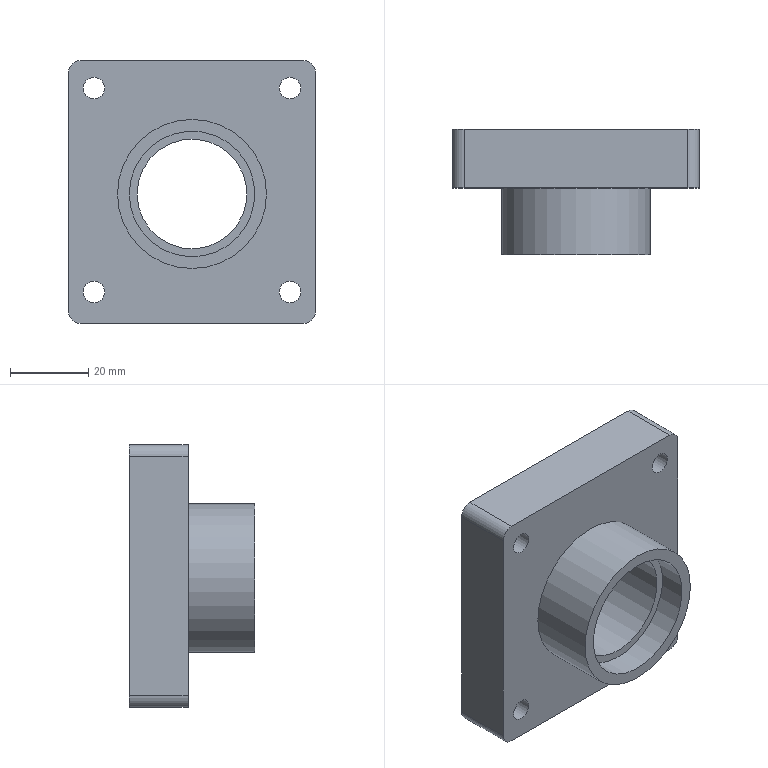Part | STEP file | ROTATION MC_NEW VER-0610_1021 | 1 solid | 29 faces | box 63 x 32 x 67 mm | volume 57913 mm3 | cylinder 16 | plane 13 | commonest cylinder face diameters 5.5 x4 6 x4 9 x4 32 x2 28 x1 38 x1
STEP:
#1=CARTESIAN_POINT('',(-200.969,622.268,-55.091));
#2=VERTEX_POINT('',#1);
#3=CARTESIAN_POINT('',(-203.969,622.268,-52.091));
#4=VERTEX_POINT('',#3);
#5=CARTESIAN_POINT('',(-203.969,622.268,-55.091));
#6=DIRECTION('',(0.,-1.,0.));
#7=DIRECTION('',(0.7071,0.,0.7071));
#8=AXIS2_PLACEMENT_3D('',#5,#6,#7);
#9=CIRCLE('',#8,3.);
#10=EDGE_CURVE('',#2,#4,#9,.T.);
#11=ORIENTED_EDGE('',*,*,#10,.T.);
#12=CARTESIAN_POINT('',(-203.969,607.268,-52.091));
#13=VERTEX_POINT('',#12);
#14=CARTESIAN_POINT('',(-203.969,604.268,-52.091));
#15=DIRECTION('',(0.,-1.,0.));
#16=VECTOR('',#15,10.);
#17=LINE('',#14,#16);
#18=EDGE_CURVE('',#4,#13,#17,.T.);
#19=ORIENTED_EDGE('',*,*,#18,.T.);
#20=CARTESIAN_POINT('',(-200.969,607.268,-55.091));
#21=VERTEX_POINT('',#20);
#22=CARTESIAN_POINT('',(-203.969,607.268,-55.091));
#23=DIRECTION('',(0.,1.,0.));
#24=DIRECTION('',(0.7071,0.,0.7071));
#25=AXIS2_PLACEMENT_3D('',#22,#23,#24);
#26=CIRCLE('',#25,3.);
#27=EDGE_CURVE('',#13,#21,#26,.T.);
#28=ORIENTED_EDGE('',*,*,#27,.T.);
#29=CARTESIAN_POINT('',(-200.969,604.268,-55.091));
#30=DIRECTION('',(0.,1.,0.));
#31=VECTOR('',#30,10.);
#32=LINE('',#29,#31);
#33=EDGE_CURVE('',#21,#2,#32,.T.);
#34=ORIENTED_EDGE('',*,*,#33,.T.);
#35=EDGE_LOOP('',(#11,#19,#28,#34));
#36=FACE_OUTER_BOUND('',#35,.T.);
#37=CARTESIAN_POINT('',(-203.969,604.268,-55.091));
#38=DIRECTION('',(0.,1.,0.));
#39=DIRECTION('',(0.7071,0.,0.7071));
#40=AXIS2_PLACEMENT_3D('',#37,#38,#39);
#41=CYLINDRICAL_SURFACE('',#40,3.);
#42=ADVANCED_FACE('',(#36),#41,.T.);
#43=ORIENTED_EDGE('',*,*,#33,.F.);
#44=CARTESIAN_POINT('',(-200.969,607.268,-116.091));
#45=VERTEX_POINT('',#44);
#46=CARTESIAN_POINT('',(-200.969,607.268,-47.091));
#47=DIRECTION('',(0.,0.,-1.));
#48=VECTOR('',#47,69.);
#49=LINE('',#46,#48);
#50=EDGE_CURVE('',#21,#45,#49,.T.);
#51=ORIENTED_EDGE('',*,*,#50,.T.);
#52=CARTESIAN_POINT('',(-200.969,622.268,-116.091));
#53=VERTEX_POINT('',#52);
#54=CARTESIAN_POINT('',(-200.969,622.268,-116.091));
#55=DIRECTION('',(0.,-1.,0.));
#56=VECTOR('',#55,10.);
#57=LINE('',#54,#56);
#58=EDGE_CURVE('',#45,#53,#57,.F.);
#59=ORIENTED_EDGE('',*,*,#58,.T.);
#60=CARTESIAN_POINT('',(-200.969,622.268,-47.091));
#61=DIRECTION('',(0.,0.,-1.));
#62=VECTOR('',#61,69.);
#63=LINE('',#60,#62);
#64=EDGE_CURVE('',#2,#53,#63,.T.);
#65=ORIENTED_EDGE('',*,*,#64,.F.);
#66=EDGE_LOOP('',(#43,#51,#59,#65));
#67=FACE_OUTER_BOUND('',#66,.T.);
#68=CARTESIAN_POINT('',(-200.969,604.268,-87.091));
#69=DIRECTION('',(1.,0.,0.));
#70=DIRECTION('',(0.,0.,-1.));
#71=AXIS2_PLACEMENT_3D('',#68,#69,#70);
#72=PLANE('',#71);
#73=ADVANCED_FACE('',(#67),#72,.T.);
#74=ORIENTED_EDGE('',*,*,#27,.F.);
#75=CARTESIAN_POINT('',(-260.969,607.268,-52.091));
#76=VERTEX_POINT('',#75);
#77=CARTESIAN_POINT('',(-260.969,607.268,-52.091));
#78=DIRECTION('',(1.,0.,0.));
#79=VECTOR('',#78,57.);
#80=LINE('',#77,#79);
#81=EDGE_CURVE('',#76,#13,#80,.T.);
#82=ORIENTED_EDGE('',*,*,#81,.F.);
#83=CARTESIAN_POINT('',(-263.969,607.268,-55.091));
#84=VERTEX_POINT('',#83);
#85=CARTESIAN_POINT('',(-260.969,607.268,-55.091));
#86=DIRECTION('',(0.,1.,0.));
#87=DIRECTION('',(-0.7071,0.,0.7071));
#88=AXIS2_PLACEMENT_3D('',#85,#86,#87);
#89=CIRCLE('',#88,3.);
#90=EDGE_CURVE('',#84,#76,#89,.T.);
#91=ORIENTED_EDGE('',*,*,#90,.F.);
#92=CARTESIAN_POINT('',(-263.969,607.268,-116.091));
#93=VERTEX_POINT('',#92);
#94=CARTESIAN_POINT('',(-263.969,607.268,-116.091));
#95=DIRECTION('',(0.,0.,1.));
#96=VECTOR('',#95,69.);
#97=LINE('',#94,#96);
#98=EDGE_CURVE('',#93,#84,#97,.T.);
#99=ORIENTED_EDGE('',*,*,#98,.F.);
#100=CARTESIAN_POINT('',(-260.969,607.268,-119.091));
#101=VERTEX_POINT('',#100);
#102=CARTESIAN_POINT('',(-260.969,607.268,-116.091));
#103=DIRECTION('',(0.,-1.,0.));
#104=DIRECTION('',(0.,0.,-1.));
#105=AXIS2_PLACEMENT_3D('',#102,#103,#104);
#106=CIRCLE('',#105,3.);
#107=EDGE_CURVE('',#93,#101,#106,.T.);
#108=ORIENTED_EDGE('',*,*,#107,.T.);
#109=CARTESIAN_POINT('',(-203.969,607.268,-119.091));
#110=VERTEX_POINT('',#109);
#111=CARTESIAN_POINT('',(-203.969,607.268,-119.091));
#112=DIRECTION('',(-1.,0.,0.));
#113=VECTOR('',#112,57.);
#114=LINE('',#111,#113);
#115=EDGE_CURVE('',#110,#101,#114,.T.);
#116=ORIENTED_EDGE('',*,*,#115,.F.);
#117=CARTESIAN_POINT('',(-203.969,607.268,-116.091));
#118=DIRECTION('',(0.,-1.,0.));
#119=DIRECTION('',(0.,0.,-1.));
#120=AXIS2_PLACEMENT_3D('',#117,#118,#119);
#121=CIRCLE('',#120,3.);
#122=EDGE_CURVE('',#110,#45,#121,.T.);
#123=ORIENTED_EDGE('',*,*,#122,.T.);
#124=ORIENTED_EDGE('',*,*,#50,.F.);
#125=EDGE_LOOP('',(#74,#82,#91,#99,#108,#116,#123,#124));
#126=FACE_OUTER_BOUND('',#125,.T.);
#127=CARTESIAN_POINT('',(-251.469,607.268,-86.091));
#128=VERTEX_POINT('',#127);
#129=CARTESIAN_POINT('',(-232.469,607.268,-86.091));
#130=DIRECTION('',(0.,1.,0.));
#131=DIRECTION('',(-1.,0.,0.));
#132=AXIS2_PLACEMENT_3D('',#129,#130,#131);
#133=CIRCLE('',#132,19.);
#134=EDGE_CURVE('',#128,#128,#133,.T.);
#135=ORIENTED_EDGE('',*,*,#134,.T.);
#136=EDGE_LOOP('',(#135));
#137=FACE_BOUND('',#136,.T.);
#138=CARTESIAN_POINT('',(-260.219,607.268,-111.091));
#139=VERTEX_POINT('',#138);
#140=CARTESIAN_POINT('',(-257.469,607.268,-111.091));
#141=DIRECTION('',(0.,-1.,0.));
#142=DIRECTION('',(-1.,0.,0.));
#143=AXIS2_PLACEMENT_3D('',#140,#141,#142);
#144=CIRCLE('',#143,2.75);
#145=EDGE_CURVE('',#139,#139,#144,.T.);
#146=ORIENTED_EDGE('',*,*,#145,.F.);
#147=EDGE_LOOP('',(#146));
#148=FACE_BOUND('',#147,.T.);
#149=CARTESIAN_POINT('',(-210.219,607.268,-59.091));
#150=VERTEX_POINT('',#149);
#151=CARTESIAN_POINT('',(-207.469,607.268,-59.091));
#152=DIRECTION('',(0.,1.,0.));
#153=DIRECTION('',(-1.,0.,0.));
#154=AXIS2_PLACEMENT_3D('',#151,#152,#153);
#155=CIRCLE('',#154,2.75);
#156=EDGE_CURVE('',#150,#150,#155,.T.);
#157=ORIENTED_EDGE('',*,*,#156,.T.);
#158=EDGE_LOOP('',(#157));
#159=FACE_BOUND('',#158,.T.);
#160=CARTESIAN_POINT('',(-260.219,607.268,-59.091));
#161=VERTEX_POINT('',#160);
#162=CARTESIAN_POINT('',(-257.469,607.268,-59.091));
#163=DIRECTION('',(0.,-1.,0.));
#164=DIRECTION('',(-1.,0.,0.));
#165=AXIS2_PLACEMENT_3D('',#162,#163,#164);
#166=CIRCLE('',#165,2.75);
#167=EDGE_CURVE('',#161,#161,#166,.T.);
#168=ORIENTED_EDGE('',*,*,#167,.F.);
#169=EDGE_LOOP('',(#168));
#170=FACE_BOUND('',#169,.T.);
#171=CARTESIAN_POINT('',(-210.219,607.268,-111.091));
#172=VERTEX_POINT('',#171);
#173=CARTESIAN_POINT('',(-207.469,607.268,-111.091));
#174=DIRECTION('',(0.,-1.,0.));
#175=DIRECTION('',(-1.,0.,0.));
#176=AXIS2_PLACEMENT_3D('',#173,#174,#175);
#177=CIRCLE('',#176,2.75);
#178=EDGE_CURVE('',#172,#172,#177,.T.);
#179=ORIENTED_EDGE('',*,*,#178,.F.);
#180=EDGE_LOOP('',(#179));
#181=FACE_BOUND('',#180,.T.);
#182=CARTESIAN_POINT('',(-232.469,607.268,-56.091));
#183=DIRECTION('',(0.,-1.,0.));
#184=DIRECTION('',(0.,0.,-1.));
#185=AXIS2_PLACEMENT_3D('',#182,#183,#184);
#186=PLANE('',#185);
#187=ADVANCED_FACE('',(#126,#137,#148,#159,#170,#181),#186,.T.);
#188=CARTESIAN_POINT('',(-260.969,622.268,-52.091));
#189=VERTEX_POINT('',#188);
#190=CARTESIAN_POINT('',(-263.969,622.268,-55.091));
#191=VERTEX_POINT('',#190);
#192=CARTESIAN_POINT('',(-260.969,622.268,-55.091));
#193=DIRECTION('',(0.,-1.,0.));
#194=DIRECTION('',(-0.7071,0.,0.7071));
#195=AXIS2_PLACEMENT_3D('',#192,#193,#194);
#196=CIRCLE('',#195,3.);
#197=EDGE_CURVE('',#189,#191,#196,.T.);
#198=ORIENTED_EDGE('',*,*,#197,.T.);
#199=CARTESIAN_POINT('',(-263.969,604.268,-55.091));
#200=DIRECTION('',(0.,-1.,0.));
#201=VECTOR('',#200,10.);
#202=LINE('',#199,#201);
#203=EDGE_CURVE('',#191,#84,#202,.T.);
#204=ORIENTED_EDGE('',*,*,#203,.T.);
#205=ORIENTED_EDGE('',*,*,#90,.T.);
#206=CARTESIAN_POINT('',(-260.969,604.268,-52.091));
#207=DIRECTION('',(0.,1.,0.));
#208=VECTOR('',#207,10.);
#209=LINE('',#206,#208);
#210=EDGE_CURVE('',#76,#189,#209,.T.);
#211=ORIENTED_EDGE('',*,*,#210,.T.);
#212=EDGE_LOOP('',(#198,#204,#205,#211));
#213=FACE_OUTER_BOUND('',#212,.T.);
#214=CARTESIAN_POINT('',(-260.969,604.268,-55.091));
#215=DIRECTION('',(0.,1.,0.));
#216=DIRECTION('',(-0.7071,0.,0.7071));
#217=AXIS2_PLACEMENT_3D('',#214,#215,#216);
#218=CYLINDRICAL_SURFACE('',#217,3.);
#219=ADVANCED_FACE('',(#213),#218,.T.);
#220=ORIENTED_EDGE('',*,*,#203,.F.);
#221=CARTESIAN_POINT('',(-263.969,622.268,-116.091));
#222=VERTEX_POINT('',#221);
#223=CARTESIAN_POINT('',(-263.969,622.268,-116.091));
#224=DIRECTION('',(0.,0.,1.));
#225=VECTOR('',#224,69.);
#226=LINE('',#223,#225);
#227=EDGE_CURVE('',#222,#191,#226,.T.);
#228=ORIENTED_EDGE('',*,*,#227,.F.);
#229=CARTESIAN_POINT('',(-263.969,612.268,-116.091));
#230=DIRECTION('',(0.,1.,0.));
#231=VECTOR('',#230,10.);
#232=LINE('',#229,#231);
#233=EDGE_CURVE('',#222,#93,#232,.F.);
#234=ORIENTED_EDGE('',*,*,#233,.T.);
#235=ORIENTED_EDGE('',*,*,#98,.T.);
#236=EDGE_LOOP('',(#220,#228,#234,#235));
#237=FACE_OUTER_BOUND('',#236,.T.);
#238=CARTESIAN_POINT('',(-263.969,604.268,-87.091));
#239=DIRECTION('',(-1.,0.,0.));
#240=DIRECTION('',(0.,0.,1.));
#241=AXIS2_PLACEMENT_3D('',#238,#239,#240);
#242=PLANE('',#241);
#243=ADVANCED_FACE('',(#237),#242,.T.);
#244=ORIENTED_EDGE('',*,*,#18,.F.);
#245=CARTESIAN_POINT('',(-260.969,622.268,-52.091));
#246=DIRECTION('',(1.,0.,0.));
#247=VECTOR('',#246,57.);
#248=LINE('',#245,#247);
#249=EDGE_CURVE('',#189,#4,#248,.T.);
#250=ORIENTED_EDGE('',*,*,#249,.F.);
#251=ORIENTED_EDGE('',*,*,#210,.F.);
#252=ORIENTED_EDGE('',*,*,#81,.T.);
#253=EDGE_LOOP('',(#244,#250,#251,#252));
#254=FACE_OUTER_BOUND('',#253,.T.);
#255=CARTESIAN_POINT('',(-235.583,604.268,-52.091));
#256=DIRECTION('',(0.,0.,1.));
#257=DIRECTION('',(1.,0.,0.));
#258=AXIS2_PLACEMENT_3D('',#255,#256,#257);
#259=PLANE('',#258);
#260=ADVANCED_FACE('',(#254),#259,.T.);
#261=ORIENTED_EDGE('',*,*,#134,.F.);
#262=CARTESIAN_POINT('',(-251.469,590.268,-86.091));
#263=VERTEX_POINT('',#262);
#264=CARTESIAN_POINT('',(-251.469,630.268,-86.091));
#265=DIRECTION('',(0.,-1.,0.));
#266=VECTOR('',#265,19.);
#267=LINE('',#264,#266);
#268=EDGE_CURVE('',#128,#263,#267,.T.);
#269=ORIENTED_EDGE('',*,*,#268,.T.);
#270=CARTESIAN_POINT('',(-232.469,590.268,-86.091));
#271=DIRECTION('',(0.,1.,0.));
#272=DIRECTION('',(-1.,0.,0.));
#273=AXIS2_PLACEMENT_3D('',#270,#271,#272);
#274=CIRCLE('',#273,19.);
#275=EDGE_CURVE('',#263,#263,#274,.T.);
#276=ORIENTED_EDGE('',*,*,#275,.T.);
#277=ORIENTED_EDGE('',*,*,#268,.F.);
#278=EDGE_LOOP('',(#261,#269,#276,#277));
#279=FACE_OUTER_BOUND('',#278,.T.);
#280=CARTESIAN_POINT('',(-232.469,630.268,-86.091));
#281=DIRECTION('',(0.,1.,0.));
#282=DIRECTION('',(1.,0.,0.));
#283=AXIS2_PLACEMENT_3D('',#280,#281,#282);
#284=CYLINDRICAL_SURFACE('',#283,19.);
#285=ADVANCED_FACE('',(#279),#284,.T.);
#286=CARTESIAN_POINT('',(-248.469,615.268,-86.091));
#287=VERTEX_POINT('',#286);
#288=CARTESIAN_POINT('',(-232.469,615.268,-86.091));
#289=DIRECTION('',(0.,1.,0.));
#290=DIRECTION('',(-1.,0.,0.));
#291=AXIS2_PLACEMENT_3D('',#288,#289,#290);
#292=CIRCLE('',#291,16.);
#293=EDGE_CURVE('',#287,#287,#292,.T.);
#294=ORIENTED_EDGE('',*,*,#293,.F.);
#295=CARTESIAN_POINT('',(-248.469,622.268,-86.091));
#296=VERTEX_POINT('',#295);
#297=CARTESIAN_POINT('',(-248.469,622.268,-86.091));
#298=DIRECTION('',(0.,1.,0.));
#299=VECTOR('',#298,16.);
#300=LINE('',#297,#299);
#301=EDGE_CURVE('',#287,#296,#300,.T.);
#302=ORIENTED_EDGE('',*,*,#301,.T.);
#303=CARTESIAN_POINT('',(-232.469,622.268,-86.091));
#304=DIRECTION('',(0.,1.,0.));
#305=DIRECTION('',(-1.,0.,0.));
#306=AXIS2_PLACEMENT_3D('',#303,#304,#305);
#307=CIRCLE('',#306,16.);
#308=EDGE_CURVE('',#296,#296,#307,.T.);
#309=ORIENTED_EDGE('',*,*,#308,.T.);
#310=ORIENTED_EDGE('',*,*,#301,.F.);
#311=EDGE_LOOP('',(#294,#302,#309,#310));
#312=FACE_OUTER_BOUND('',#311,.T.);
#313=CARTESIAN_POINT('',(-232.469,622.268,-86.091));
#314=DIRECTION('',(0.,1.,0.));
#315=DIRECTION('',(1.,0.,0.));
#316=AXIS2_PLACEMENT_3D('',#313,#314,#315);
#317=CYLINDRICAL_SURFACE('',#316,16.);
#318=ADVANCED_FACE('',(#312),#317,.F.);
#319=ORIENTED_EDGE('',*,*,#293,.T.);
#320=EDGE_LOOP('',(#319));
#321=FACE_OUTER_BOUND('',#320,.T.);
#322=CARTESIAN_POINT('',(-246.469,615.268,-86.091));
#323=VERTEX_POINT('',#322);
#324=CARTESIAN_POINT('',(-232.469,615.268,-86.091));
#325=DIRECTION('',(0.,1.,0.));
#326=DIRECTION('',(-1.,0.,0.));
#327=AXIS2_PLACEMENT_3D('',#324,#325,#326);
#328=CIRCLE('',#327,14.);
#329=EDGE_CURVE('',#323,#323,#328,.T.);
#330=ORIENTED_EDGE('',*,*,#329,.F.);
#331=EDGE_LOOP('',(#330));
#332=FACE_BOUND('',#331,.T.);
#333=CARTESIAN_POINT('',(-232.469,615.268,-72.091));
#334=DIRECTION('',(0.,1.,0.));
#335=DIRECTION('',(0.,0.,1.));
#336=AXIS2_PLACEMENT_3D('',#333,#334,#335);
#337=PLANE('',#336);
#338=ADVANCED_FACE('',(#321,#332),#337,.T.);
#339=CARTESIAN_POINT('',(-246.469,597.268,-86.091));
#340=VERTEX_POINT('',#339);
#341=CARTESIAN_POINT('',(-232.469,597.268,-86.091));
#342=DIRECTION('',(0.,1.,0.));
#343=DIRECTION('',(-1.,0.,0.));
#344=AXIS2_PLACEMENT_3D('',#341,#342,#343);
#345=CIRCLE('',#344,14.);
#346=EDGE_CURVE('',#340,#340,#345,.T.);
#347=ORIENTED_EDGE('',*,*,#346,.F.);
#348=CARTESIAN_POINT('',(-246.469,630.268,-86.091));
#349=DIRECTION('',(0.,1.,0.));
#350=VECTOR('',#349,14.);
#351=LINE('',#348,#350);
#352=EDGE_CURVE('',#340,#323,#351,.T.);
#353=ORIENTED_EDGE('',*,*,#352,.T.);
#354=ORIENTED_EDGE('',*,*,#329,.T.);
#355=ORIENTED_EDGE('',*,*,#352,.F.);
#356=EDGE_LOOP('',(#347,#353,#354,#355));
#357=FACE_OUTER_BOUND('',#356,.T.);
#358=CARTESIAN_POINT('',(-232.469,630.268,-86.091));
#359=DIRECTION('',(0.,1.,0.));
#360=DIRECTION('',(1.,0.,0.));
#361=AXIS2_PLACEMENT_3D('',#358,#359,#360);
#362=CYLINDRICAL_SURFACE('',#361,14.);
#363=ADVANCED_FACE('',(#357),#362,.F.);
#364=CARTESIAN_POINT('',(-248.469,597.268,-86.091));
#365=VERTEX_POINT('',#364);
#366=CARTESIAN_POINT('',(-232.469,597.268,-86.091));
#367=DIRECTION('',(0.,1.,0.));
#368=DIRECTION('',(-1.,0.,0.));
#369=AXIS2_PLACEMENT_3D('',#366,#367,#368);
#370=CIRCLE('',#369,16.);
#371=EDGE_CURVE('',#365,#365,#370,.T.);
#372=ORIENTED_EDGE('',*,*,#371,.F.);
#373=EDGE_LOOP('',(#372));
#374=FACE_OUTER_BOUND('',#373,.T.);
#375=ORIENTED_EDGE('',*,*,#346,.T.);
#376=EDGE_LOOP('',(#375));
#377=FACE_BOUND('',#376,.T.);
#378=CARTESIAN_POINT('',(-232.469,597.268,-70.091));
#379=DIRECTION('',(0.,-1.,0.));
#380=DIRECTION('',(0.,0.,-1.));
#381=AXIS2_PLACEMENT_3D('',#378,#379,#380);
#382=PLANE('',#381);
#383=ADVANCED_FACE('',(#374,#377),#382,.T.);
#384=CARTESIAN_POINT('',(-248.469,590.268,-86.091));
#385=VERTEX_POINT('',#384);
#386=CARTESIAN_POINT('',(-232.469,590.268,-86.091));
#387=DIRECTION('',(0.,1.,0.));
#388=DIRECTION('',(-1.,0.,0.));
#389=AXIS2_PLACEMENT_3D('',#386,#387,#388);
#390=CIRCLE('',#389,16.);
#391=EDGE_CURVE('',#385,#385,#390,.T.);
#392=ORIENTED_EDGE('',*,*,#391,.F.);
#393=CARTESIAN_POINT('',(-248.469,630.268,-86.091));
#394=DIRECTION('',(0.,1.,0.));
#395=VECTOR('',#394,16.);
#396=LINE('',#393,#395);
#397=EDGE_CURVE('',#385,#365,#396,.T.);
#398=ORIENTED_EDGE('',*,*,#397,.T.);
#399=ORIENTED_EDGE('',*,*,#371,.T.);
#400=ORIENTED_EDGE('',*,*,#397,.F.);
#401=EDGE_LOOP('',(#392,#398,#399,#400));
#402=FACE_OUTER_BOUND('',#401,.T.);
#403=CARTESIAN_POINT('',(-232.469,630.268,-86.091));
#404=DIRECTION('',(0.,1.,0.));
#405=DIRECTION('',(1.,0.,0.));
#406=AXIS2_PLACEMENT_3D('',#403,#404,#405);
#407=CYLINDRICAL_SURFACE('',#406,16.);
#408=ADVANCED_FACE('',(#402),#407,.F.);
#409=ORIENTED_EDGE('',*,*,#275,.F.);
#410=EDGE_LOOP('',(#409));
#411=FACE_OUTER_BOUND('',#410,.T.);
#412=ORIENTED_EDGE('',*,*,#391,.T.);
#413=EDGE_LOOP('',(#412));
#414=FACE_BOUND('',#413,.T.);
#415=CARTESIAN_POINT('',(-232.469,590.268,-67.091));
#416=DIRECTION('',(0.,-1.,0.));
#417=DIRECTION('',(0.,0.,-1.));
#418=AXIS2_PLACEMENT_3D('',#415,#416,#417);
#419=PLANE('',#418);
#420=ADVANCED_FACE('',(#411,#414),#419,.T.);
#421=ORIENTED_EDGE('',*,*,#115,.T.);
#422=CARTESIAN_POINT('',(-260.969,622.268,-119.091));
#423=VERTEX_POINT('',#422);
#424=CARTESIAN_POINT('',(-260.969,612.268,-119.091));
#425=DIRECTION('',(0.,1.,0.));
#426=VECTOR('',#425,10.);
#427=LINE('',#424,#426);
#428=EDGE_CURVE('',#101,#423,#427,.T.);
#429=ORIENTED_EDGE('',*,*,#428,.T.);
#430=CARTESIAN_POINT('',(-203.969,622.268,-119.091));
#431=VERTEX_POINT('',#430);
#432=CARTESIAN_POINT('',(-203.969,622.268,-119.091));
#433=DIRECTION('',(-1.,0.,0.));
#434=VECTOR('',#433,57.);
#435=LINE('',#432,#434);
#436=EDGE_CURVE('',#431,#423,#435,.T.);
#437=ORIENTED_EDGE('',*,*,#436,.F.);
#438=CARTESIAN_POINT('',(-203.969,622.268,-119.091));
#439=DIRECTION('',(0.,-1.,0.));
#440=VECTOR('',#439,10.);
#441=LINE('',#438,#440);
#442=EDGE_CURVE('',#431,#110,#441,.T.);
#443=ORIENTED_EDGE('',*,*,#442,.T.);
#444=EDGE_LOOP('',(#421,#429,#437,#443));
#445=FACE_OUTER_BOUND('',#444,.T.);
#446=CARTESIAN_POINT('',(-235.583,604.268,-119.091));
#447=DIRECTION('',(0.,0.,-1.));
#448=DIRECTION('',(-1.,0.,0.));
#449=AXIS2_PLACEMENT_3D('',#446,#447,#448);
#450=PLANE('',#449);
#451=ADVANCED_FACE('',(#445),#450,.T.);
#452=ORIENTED_EDGE('',*,*,#10,.F.);
#453=ORIENTED_EDGE('',*,*,#64,.T.);
#454=CARTESIAN_POINT('',(-203.969,622.268,-116.091));
#455=DIRECTION('',(0.,1.,0.));
#456=DIRECTION('',(0.,0.,1.));
#457=AXIS2_PLACEMENT_3D('',#454,#455,#456);
#458=CIRCLE('',#457,3.);
#459=EDGE_CURVE('',#53,#431,#458,.T.);
#460=ORIENTED_EDGE('',*,*,#459,.T.);
#461=ORIENTED_EDGE('',*,*,#436,.T.);
#462=CARTESIAN_POINT('',(-260.969,622.268,-116.091));
#463=DIRECTION('',(0.,1.,0.));
#464=DIRECTION('',(0.,0.,1.));
#465=AXIS2_PLACEMENT_3D('',#462,#463,#464);
#466=CIRCLE('',#465,3.);
#467=EDGE_CURVE('',#423,#222,#466,.T.);
#468=ORIENTED_EDGE('',*,*,#467,.T.);
#469=ORIENTED_EDGE('',*,*,#227,.T.);
#470=ORIENTED_EDGE('',*,*,#197,.F.);
#471=ORIENTED_EDGE('',*,*,#249,.T.);
#472=EDGE_LOOP('',(#452,#453,#460,#461,#468,#469,#470,#471));
#473=FACE_OUTER_BOUND('',#472,.T.);
#474=CARTESIAN_POINT('',(-257.469,622.268,-106.591));
#475=VERTEX_POINT('',#474);
#476=CARTESIAN_POINT('',(-257.469,622.268,-115.591));
#477=VERTEX_POINT('',#476);
#478=CARTESIAN_POINT('',(-257.469,622.268,-111.091));
#479=DIRECTION('',(0.,1.,0.));
#480=DIRECTION('',(0.,0.,1.));
#481=AXIS2_PLACEMENT_3D('',#478,#479,#480);
#482=CIRCLE('',#481,4.5);
#483=EDGE_CURVE('',#475,#477,#482,.F.);
#484=ORIENTED_EDGE('',*,*,#483,.T.);
#485=CARTESIAN_POINT('',(-257.469,622.268,-111.091));
#486=DIRECTION('',(0.,1.,0.));
#487=DIRECTION('',(0.,0.,1.));
#488=AXIS2_PLACEMENT_3D('',#485,#486,#487);
#489=CIRCLE('',#488,4.5);
#490=EDGE_CURVE('',#477,#475,#489,.F.);
#491=ORIENTED_EDGE('',*,*,#490,.T.);
#492=EDGE_LOOP('',(#484,#491));
#493=FACE_BOUND('',#492,.T.);
#494=CARTESIAN_POINT('',(-207.469,622.268,-54.591));
#495=VERTEX_POINT('',#494);
#496=CARTESIAN_POINT('',(-207.469,622.268,-63.591));
#497=VERTEX_POINT('',#496);
#498=CARTESIAN_POINT('',(-207.469,622.268,-59.091));
#499=DIRECTION('',(0.,1.,0.));
#500=DIRECTION('',(0.,0.,1.));
#501=AXIS2_PLACEMENT_3D('',#498,#499,#500);
#502=CIRCLE('',#501,4.5);
#503=EDGE_CURVE('',#495,#497,#502,.F.);
#504=ORIENTED_EDGE('',*,*,#503,.T.);
#505=CARTESIAN_POINT('',(-207.469,622.268,-59.091));
#506=DIRECTION('',(0.,1.,0.));
#507=DIRECTION('',(0.,0.,1.));
#508=AXIS2_PLACEMENT_3D('',#505,#506,#507);
#509=CIRCLE('',#508,4.5);
#510=EDGE_CURVE('',#497,#495,#509,.F.);
#511=ORIENTED_EDGE('',*,*,#510,.T.);
#512=EDGE_LOOP('',(#504,#511));
#513=FACE_BOUND('',#512,.T.);
#514=CARTESIAN_POINT('',(-257.469,622.268,-54.591));
#515=VERTEX_POINT('',#514);
#516=CARTESIAN_POINT('',(-257.469,622.268,-63.591));
#517=VERTEX_POINT('',#516);
#518=CARTESIAN_POINT('',(-257.469,622.268,-59.091));
#519=DIRECTION('',(0.,1.,0.));
#520=DIRECTION('',(0.,0.,1.));
#521=AXIS2_PLACEMENT_3D('',#518,#519,#520);
#522=CIRCLE('',#521,4.5);
#523=EDGE_CURVE('',#515,#517,#522,.F.);
#524=ORIENTED_EDGE('',*,*,#523,.T.);
#525=CARTESIAN_POINT('',(-257.469,622.268,-59.091));
#526=DIRECTION('',(0.,1.,0.));
#527=DIRECTION('',(0.,0.,1.));
#528=AXIS2_PLACEMENT_3D('',#525,#526,#527);
#529=CIRCLE('',#528,4.5);
#530=EDGE_CURVE('',#517,#515,#529,.F.);
#531=ORIENTED_EDGE('',*,*,#530,.T.);
#532=EDGE_LOOP('',(#524,#531));
#533=FACE_BOUND('',#532,.T.);
#534=CARTESIAN_POINT('',(-207.469,622.268,-106.591));
#535=VERTEX_POINT('',#534);
#536=CARTESIAN_POINT('',(-210.651,622.268,-114.273));
#537=VERTEX_POINT('',#536);
#538=CARTESIAN_POINT('',(-207.469,622.268,-111.091));
#539=DIRECTION('',(0.,1.,0.));
#540=DIRECTION('',(0.,0.,1.));
#541=AXIS2_PLACEMENT_3D('',#538,#539,#540);
#542=CIRCLE('',#541,4.5);
#543=EDGE_CURVE('',#535,#537,#542,.F.);
#544=ORIENTED_EDGE('',*,*,#543,.T.);
#545=CARTESIAN_POINT('',(-207.469,622.268,-111.091));
#546=DIRECTION('',(0.,1.,0.));
#547=DIRECTION('',(0.,0.,1.));
#548=AXIS2_PLACEMENT_3D('',#545,#546,#547);
#549=CIRCLE('',#548,4.5);
#550=EDGE_CURVE('',#537,#535,#549,.F.);
#551=ORIENTED_EDGE('',*,*,#550,.T.);
#552=EDGE_LOOP('',(#544,#551));
#553=FACE_BOUND('',#552,.T.);
#554=ORIENTED_EDGE('',*,*,#308,.F.);
#555=EDGE_LOOP('',(#554));
#556=FACE_BOUND('',#555,.T.);
#557=CARTESIAN_POINT('',(-232.469,622.268,-70.091));
#558=DIRECTION('',(0.,1.,0.));
#559=DIRECTION('',(0.,0.,1.));
#560=AXIS2_PLACEMENT_3D('',#557,#558,#559);
#561=PLANE('',#560);
#562=ADVANCED_FACE('',(#473,#493,#513,#533,#553,#556),#561,.T.);
#563=CARTESIAN_POINT('',(-211.969,617.268,-111.091));
#564=VERTEX_POINT('',#563);
#565=CARTESIAN_POINT('',(-210.651,617.268,-114.273));
#566=VERTEX_POINT('',#565);
#567=CARTESIAN_POINT('',(-207.469,617.268,-111.091));
#568=DIRECTION('',(0.,-1.,0.));
#569=DIRECTION('',(-1.,0.,0.));
#570=AXIS2_PLACEMENT_3D('',#567,#568,#569);
#571=CIRCLE('',#570,4.5);
#572=EDGE_CURVE('',#564,#566,#571,.F.);
#573=ORIENTED_EDGE('',*,*,#572,.F.);
#574=CARTESIAN_POINT('',(-207.469,617.268,-111.091));
#575=DIRECTION('',(0.,-1.,0.));
#576=DIRECTION('',(-1.,0.,0.));
#577=AXIS2_PLACEMENT_3D('',#574,#575,#576);
#578=CIRCLE('',#577,4.5);
#579=EDGE_CURVE('',#566,#564,#578,.F.);
#580=ORIENTED_EDGE('',*,*,#579,.F.);
#581=CARTESIAN_POINT('',(-210.651,612.268,-114.273));
#582=DIRECTION('',(0.,1.,0.));
#583=VECTOR('',#582,4.5);
#584=LINE('',#581,#583);
#585=EDGE_CURVE('',#566,#537,#584,.T.);
#586=ORIENTED_EDGE('',*,*,#585,.T.);
#587=ORIENTED_EDGE('',*,*,#543,.F.);
#588=ORIENTED_EDGE('',*,*,#550,.F.);
#589=ORIENTED_EDGE('',*,*,#585,.F.);
#590=EDGE_LOOP('',(#573,#580,#586,#587,#588,#589));
#591=FACE_OUTER_BOUND('',#590,.T.);
#592=CARTESIAN_POINT('',(-207.469,612.268,-111.091));
#593=DIRECTION('',(0.,1.,0.));
#594=DIRECTION('',(0.7071,0.,0.7071));
#595=AXIS2_PLACEMENT_3D('',#592,#593,#594);
#596=CYLINDRICAL_SURFACE('',#595,4.5);
#597=ADVANCED_FACE('',(#591),#596,.F.);
#598=ORIENTED_EDGE('',*,*,#178,.T.);
#599=CARTESIAN_POINT('',(-210.219,617.268,-111.091));
#600=VERTEX_POINT('',#599);
#601=CARTESIAN_POINT('',(-210.219,622.268,-111.091));
#602=DIRECTION('',(0.,1.,0.));
#603=VECTOR('',#602,2.75);
#604=LINE('',#601,#603);
#605=EDGE_CURVE('',#172,#600,#604,.T.);
#606=ORIENTED_EDGE('',*,*,#605,.T.);
#607=CARTESIAN_POINT('',(-207.469,617.268,-111.091));
#608=DIRECTION('',(0.,1.,0.));
#609=DIRECTION('',(-1.,0.,0.));
#610=AXIS2_PLACEMENT_3D('',#607,#608,#609);
#611=CIRCLE('',#610,2.75);
#612=EDGE_CURVE('',#600,#600,#611,.T.);
#613=ORIENTED_EDGE('',*,*,#612,.T.);
#614=ORIENTED_EDGE('',*,*,#605,.F.);
#615=EDGE_LOOP('',(#598,#606,#613,#614));
#616=FACE_OUTER_BOUND('',#615,.T.);
#617=CARTESIAN_POINT('',(-207.469,622.268,-111.091));
#618=DIRECTION('',(0.,1.,0.));
#619=DIRECTION('',(1.,0.,0.));
#620=AXIS2_PLACEMENT_3D('',#617,#618,#619);
#621=CYLINDRICAL_SURFACE('',#620,2.75);
#622=ADVANCED_FACE('',(#616),#621,.F.);
#623=ORIENTED_EDGE('',*,*,#572,.T.);
#624=ORIENTED_EDGE('',*,*,#579,.T.);
#625=EDGE_LOOP('',(#623,#624));
#626=FACE_OUTER_BOUND('',#625,.T.);
#627=ORIENTED_EDGE('',*,*,#612,.F.);
#628=EDGE_LOOP('',(#627));
#629=FACE_BOUND('',#628,.T.);
#630=CARTESIAN_POINT('',(-204.969,617.268,-100.531));
#631=DIRECTION('',(0.,1.,0.));
#632=DIRECTION('',(0.,0.,1.));
#633=AXIS2_PLACEMENT_3D('',#630,#631,#632);
#634=PLANE('',#633);
#635=ADVANCED_FACE('',(#626,#629),#634,.T.);
#636=CARTESIAN_POINT('',(-261.969,617.268,-59.091));
#637=VERTEX_POINT('',#636);
#638=CARTESIAN_POINT('',(-257.469,617.268,-63.591));
#639=VERTEX_POINT('',#638);
#640=CARTESIAN_POINT('',(-257.469,617.268,-59.091));
#641=DIRECTION('',(0.,-1.,0.));
#642=DIRECTION('',(-1.,0.,0.));
#643=AXIS2_PLACEMENT_3D('',#640,#641,#642);
#644=CIRCLE('',#643,4.5);
#645=EDGE_CURVE('',#637,#639,#644,.F.);
#646=ORIENTED_EDGE('',*,*,#645,.F.);
#647=CARTESIAN_POINT('',(-257.469,617.268,-59.091));
#648=DIRECTION('',(0.,-1.,0.));
#649=DIRECTION('',(-1.,0.,0.));
#650=AXIS2_PLACEMENT_3D('',#647,#648,#649);
#651=CIRCLE('',#650,4.5);
#652=EDGE_CURVE('',#639,#637,#651,.F.);
#653=ORIENTED_EDGE('',*,*,#652,.F.);
#654=CARTESIAN_POINT('',(-257.469,612.268,-63.591));
#655=DIRECTION('',(0.,1.,0.));
#656=VECTOR('',#655,4.5);
#657=LINE('',#654,#656);
#658=EDGE_CURVE('',#639,#517,#657,.T.);
#659=ORIENTED_EDGE('',*,*,#658,.T.);
#660=ORIENTED_EDGE('',*,*,#523,.F.);
#661=ORIENTED_EDGE('',*,*,#530,.F.);
#662=ORIENTED_EDGE('',*,*,#658,.F.);
#663=EDGE_LOOP('',(#646,#653,#659,#660,#661,#662));
#664=FACE_OUTER_BOUND('',#663,.T.);
#665=CARTESIAN_POINT('',(-257.469,612.268,-59.091));
#666=DIRECTION('',(0.,1.,0.));
#667=DIRECTION('',(0.,0.,1.));
#668=AXIS2_PLACEMENT_3D('',#665,#666,#667);
#669=CYLINDRICAL_SURFACE('',#668,4.5);
#670=ADVANCED_FACE('',(#664),#669,.F.);
#671=ORIENTED_EDGE('',*,*,#167,.T.);
#672=CARTESIAN_POINT('',(-260.219,617.268,-59.091));
#673=VERTEX_POINT('',#672);
#674=CARTESIAN_POINT('',(-260.219,622.268,-59.091));
#675=DIRECTION('',(0.,1.,0.));
#676=VECTOR('',#675,2.75);
#677=LINE('',#674,#676);
#678=EDGE_CURVE('',#161,#673,#677,.T.);
#679=ORIENTED_EDGE('',*,*,#678,.T.);
#680=CARTESIAN_POINT('',(-257.469,617.268,-59.091));
#681=DIRECTION('',(0.,1.,0.));
#682=DIRECTION('',(-1.,0.,0.));
#683=AXIS2_PLACEMENT_3D('',#680,#681,#682);
#684=CIRCLE('',#683,2.75);
#685=EDGE_CURVE('',#673,#673,#684,.T.);
#686=ORIENTED_EDGE('',*,*,#685,.T.);
#687=ORIENTED_EDGE('',*,*,#678,.F.);
#688=EDGE_LOOP('',(#671,#679,#686,#687));
#689=FACE_OUTER_BOUND('',#688,.T.);
#690=CARTESIAN_POINT('',(-257.469,622.268,-59.091));
#691=DIRECTION('',(0.,1.,0.));
#692=DIRECTION('',(1.,0.,0.));
#693=AXIS2_PLACEMENT_3D('',#690,#691,#692);
#694=CYLINDRICAL_SURFACE('',#693,2.75);
#695=ADVANCED_FACE('',(#689),#694,.F.);
#696=ORIENTED_EDGE('',*,*,#645,.T.);
#697=ORIENTED_EDGE('',*,*,#652,.T.);
#698=EDGE_LOOP('',(#696,#697));
#699=FACE_OUTER_BOUND('',#698,.T.);
#700=ORIENTED_EDGE('',*,*,#685,.F.);
#701=EDGE_LOOP('',(#700));
#702=FACE_BOUND('',#701,.T.);
#703=CARTESIAN_POINT('',(-266.839,617.268,-79.091));
#704=DIRECTION('',(0.,1.,0.));
#705=DIRECTION('',(0.,0.,1.));
#706=AXIS2_PLACEMENT_3D('',#703,#704,#705);
#707=PLANE('',#706);
#708=ADVANCED_FACE('',(#699,#702),#707,.T.);
#709=CARTESIAN_POINT('',(-211.969,617.268,-59.091));
#710=VERTEX_POINT('',#709);
#711=CARTESIAN_POINT('',(-207.469,617.268,-63.591));
#712=VERTEX_POINT('',#711);
#713=CARTESIAN_POINT('',(-207.469,617.268,-59.091));
#714=DIRECTION('',(0.,-1.,0.));
#715=DIRECTION('',(-1.,0.,0.));
#716=AXIS2_PLACEMENT_3D('',#713,#714,#715);
#717=CIRCLE('',#716,4.5);
#718=EDGE_CURVE('',#710,#712,#717,.F.);
#719=ORIENTED_EDGE('',*,*,#718,.F.);
#720=CARTESIAN_POINT('',(-207.469,617.268,-59.091));
#721=DIRECTION('',(0.,-1.,0.));
#722=DIRECTION('',(-1.,0.,0.));
#723=AXIS2_PLACEMENT_3D('',#720,#721,#722);
#724=CIRCLE('',#723,4.5);
#725=EDGE_CURVE('',#712,#710,#724,.F.);
#726=ORIENTED_EDGE('',*,*,#725,.F.);
#727=CARTESIAN_POINT('',(-207.469,612.268,-63.591));
#728=DIRECTION('',(0.,1.,0.));
#729=VECTOR('',#728,4.5);
#730=LINE('',#727,#729);
#731=EDGE_CURVE('',#712,#497,#730,.T.);
#732=ORIENTED_EDGE('',*,*,#731,.T.);
#733=ORIENTED_EDGE('',*,*,#503,.F.);
#734=ORIENTED_EDGE('',*,*,#510,.F.);
#735=ORIENTED_EDGE('',*,*,#731,.F.);
#736=EDGE_LOOP('',(#719,#726,#732,#733,#734,#735));
#737=FACE_OUTER_BOUND('',#736,.T.);
#738=CARTESIAN_POINT('',(-207.469,612.268,-59.091));
#739=DIRECTION('',(0.,1.,0.));
#740=DIRECTION('',(0.,0.,1.));
#741=AXIS2_PLACEMENT_3D('',#738,#739,#740);
#742=CYLINDRICAL_SURFACE('',#741,4.5);
#743=ADVANCED_FACE('',(#737),#742,.F.);
#744=ORIENTED_EDGE('',*,*,#156,.F.);
#745=CARTESIAN_POINT('',(-210.219,617.268,-59.091));
#746=VERTEX_POINT('',#745);
#747=CARTESIAN_POINT('',(-210.219,622.268,-59.091));
#748=DIRECTION('',(0.,1.,0.));
#749=VECTOR('',#748,2.75);
#750=LINE('',#747,#749);
#751=EDGE_CURVE('',#150,#746,#750,.T.);
#752=ORIENTED_EDGE('',*,*,#751,.T.);
#753=CARTESIAN_POINT('',(-207.469,617.268,-59.091));
#754=DIRECTION('',(0.,-1.,0.));
#755=DIRECTION('',(-1.,0.,0.));
#756=AXIS2_PLACEMENT_3D('',#753,#754,#755);
#757=CIRCLE('',#756,2.75);
#758=EDGE_CURVE('',#746,#746,#757,.T.);
#759=ORIENTED_EDGE('',*,*,#758,.F.);
#760=ORIENTED_EDGE('',*,*,#751,.F.);
#761=EDGE_LOOP('',(#744,#752,#759,#760));
#762=FACE_OUTER_BOUND('',#761,.T.);
#763=CARTESIAN_POINT('',(-207.469,622.268,-59.091));
#764=DIRECTION('',(0.,1.,0.));
#765=DIRECTION('',(1.,0.,0.));
#766=AXIS2_PLACEMENT_3D('',#763,#764,#765);
#767=CYLINDRICAL_SURFACE('',#766,2.75);
#768=ADVANCED_FACE('',(#762),#767,.F.);
#769=ORIENTED_EDGE('',*,*,#718,.T.);
#770=ORIENTED_EDGE('',*,*,#725,.T.);
#771=EDGE_LOOP('',(#769,#770));
#772=FACE_OUTER_BOUND('',#771,.T.);
#773=ORIENTED_EDGE('',*,*,#758,.T.);
#774=EDGE_LOOP('',(#773));
#775=FACE_BOUND('',#774,.T.);
#776=CARTESIAN_POINT('',(-204.969,617.268,-79.091));
#777=DIRECTION('',(0.,1.,0.));
#778=DIRECTION('',(0.,0.,1.));
#779=AXIS2_PLACEMENT_3D('',#776,#777,#778);
#780=PLANE('',#779);
#781=ADVANCED_FACE('',(#772,#775),#780,.T.);
#782=CARTESIAN_POINT('',(-261.969,617.268,-111.091));
#783=VERTEX_POINT('',#782);
#784=CARTESIAN_POINT('',(-257.469,617.268,-115.591));
#785=VERTEX_POINT('',#784);
#786=CARTESIAN_POINT('',(-257.469,617.268,-111.091));
#787=DIRECTION('',(0.,-1.,0.));
#788=DIRECTION('',(-1.,0.,0.));
#789=AXIS2_PLACEMENT_3D('',#786,#787,#788);
#790=CIRCLE('',#789,4.5);
#791=EDGE_CURVE('',#783,#785,#790,.F.);
#792=ORIENTED_EDGE('',*,*,#791,.F.);
#793=CARTESIAN_POINT('',(-257.469,617.268,-111.091));
#794=DIRECTION('',(0.,-1.,0.));
#795=DIRECTION('',(-1.,0.,0.));
#796=AXIS2_PLACEMENT_3D('',#793,#794,#795);
#797=CIRCLE('',#796,4.5);
#798=EDGE_CURVE('',#785,#783,#797,.F.);
#799=ORIENTED_EDGE('',*,*,#798,.F.);
#800=CARTESIAN_POINT('',(-257.469,612.268,-115.591));
#801=DIRECTION('',(0.,1.,0.));
#802=VECTOR('',#801,4.5);
#803=LINE('',#800,#802);
#804=EDGE_CURVE('',#785,#477,#803,.T.);
#805=ORIENTED_EDGE('',*,*,#804,.T.);
#806=ORIENTED_EDGE('',*,*,#483,.F.);
#807=ORIENTED_EDGE('',*,*,#490,.F.);
#808=ORIENTED_EDGE('',*,*,#804,.F.);
#809=EDGE_LOOP('',(#792,#799,#805,#806,#807,#808));
#810=FACE_OUTER_BOUND('',#809,.T.);
#811=CARTESIAN_POINT('',(-257.469,612.268,-111.091));
#812=DIRECTION('',(0.,1.,0.));
#813=DIRECTION('',(0.,0.,1.));
#814=AXIS2_PLACEMENT_3D('',#811,#812,#813);
#815=CYLINDRICAL_SURFACE('',#814,4.5);
#816=ADVANCED_FACE('',(#810),#815,.F.);
#817=ORIENTED_EDGE('',*,*,#145,.T.);
#818=CARTESIAN_POINT('',(-260.219,617.268,-111.091));
#819=VERTEX_POINT('',#818);
#820=CARTESIAN_POINT('',(-260.219,622.268,-111.091));
#821=DIRECTION('',(0.,1.,0.));
#822=VECTOR('',#821,2.75);
#823=LINE('',#820,#822);
#824=EDGE_CURVE('',#139,#819,#823,.T.);
#825=ORIENTED_EDGE('',*,*,#824,.T.);
#826=CARTESIAN_POINT('',(-257.469,617.268,-111.091));
#827=DIRECTION('',(0.,1.,0.));
#828=DIRECTION('',(-1.,0.,0.));
#829=AXIS2_PLACEMENT_3D('',#826,#827,#828);
#830=CIRCLE('',#829,2.75);
#831=EDGE_CURVE('',#819,#819,#830,.T.);
#832=ORIENTED_EDGE('',*,*,#831,.T.);
#833=ORIENTED_EDGE('',*,*,#824,.F.);
#834=EDGE_LOOP('',(#817,#825,#832,#833));
#835=FACE_OUTER_BOUND('',#834,.T.);
#836=CARTESIAN_POINT('',(-257.469,622.268,-111.091));
#837=DIRECTION('',(0.,1.,0.));
#838=DIRECTION('',(1.,0.,0.));
#839=AXIS2_PLACEMENT_3D('',#836,#837,#838);
#840=CYLINDRICAL_SURFACE('',#839,2.75);
#841=ADVANCED_FACE('',(#835),#840,.F.);
#842=ORIENTED_EDGE('',*,*,#791,.T.);
#843=ORIENTED_EDGE('',*,*,#798,.T.);
#844=EDGE_LOOP('',(#842,#843));
#845=FACE_OUTER_BOUND('',#844,.T.);
#846=ORIENTED_EDGE('',*,*,#831,.F.);
#847=EDGE_LOOP('',(#846));
#848=FACE_BOUND('',#847,.T.);
#849=CARTESIAN_POINT('',(-266.839,617.268,-100.531));
#850=DIRECTION('',(0.,1.,0.));
#851=DIRECTION('',(0.,0.,1.));
#852=AXIS2_PLACEMENT_3D('',#849,#850,#851);
#853=PLANE('',#852);
#854=ADVANCED_FACE('',(#845,#848),#853,.T.);
#855=ORIENTED_EDGE('',*,*,#459,.F.);
#856=ORIENTED_EDGE('',*,*,#58,.F.);
#857=ORIENTED_EDGE('',*,*,#122,.F.);
#858=ORIENTED_EDGE('',*,*,#442,.F.);
#859=EDGE_LOOP('',(#855,#856,#857,#858));
#860=FACE_OUTER_BOUND('',#859,.T.);
#861=CARTESIAN_POINT('',(-203.969,604.268,-116.091));
#862=DIRECTION('',(0.,-1.,0.));
#863=DIRECTION('',(0.,0.,-1.));
#864=AXIS2_PLACEMENT_3D('',#861,#862,#863);
#865=CYLINDRICAL_SURFACE('',#864,3.);
#866=ADVANCED_FACE('',(#860),#865,.T.);
#867=ORIENTED_EDGE('',*,*,#107,.F.);
#868=ORIENTED_EDGE('',*,*,#233,.F.);
#869=ORIENTED_EDGE('',*,*,#467,.F.);
#870=ORIENTED_EDGE('',*,*,#428,.F.);
#871=EDGE_LOOP('',(#867,#868,#869,#870));
#872=FACE_OUTER_BOUND('',#871,.T.);
#873=CARTESIAN_POINT('',(-260.969,604.268,-116.091));
#874=DIRECTION('',(0.,1.,0.));
#875=DIRECTION('',(0.,0.,1.));
#876=AXIS2_PLACEMENT_3D('',#873,#874,#875);
#877=CYLINDRICAL_SURFACE('',#876,3.);
#878=ADVANCED_FACE('',(#872),#877,.T.);
#879=CLOSED_SHELL('',(#42,#73,#187,#219,#243,#260,#285,#318,#338,#363,#383,#408,#420,#451,#562,#597,#622,#635,#670,#695,#708,#743,#768,#781,#816,#841,#854,#866,#878));
#880=MANIFOLD_SOLID_BREP('',#879);
#881=(LENGTH_UNIT()NAMED_UNIT(*)SI_UNIT(.MILLI.,.METRE.));
#882=UNCERTAINTY_MEASURE_WITH_UNIT(LENGTH_MEASURE(0.01),#881,'','');
#883=(NAMED_UNIT(*)PLANE_ANGLE_UNIT()SI_UNIT($,.RADIAN.));
#884=(NAMED_UNIT(*)SI_UNIT($,.STERADIAN.)SOLID_ANGLE_UNIT());
#885=(GEOMETRIC_REPRESENTATION_CONTEXT(3)GLOBAL_UNCERTAINTY_ASSIGNED_CONTEXT((#882))GLOBAL_UNIT_ASSIGNED_CONTEXT((#881,#883,#884))REPRESENTATION_CONTEXT('',''));
#886=ADVANCED_BREP_SHAPE_REPRESENTATION('',(#880),#885);